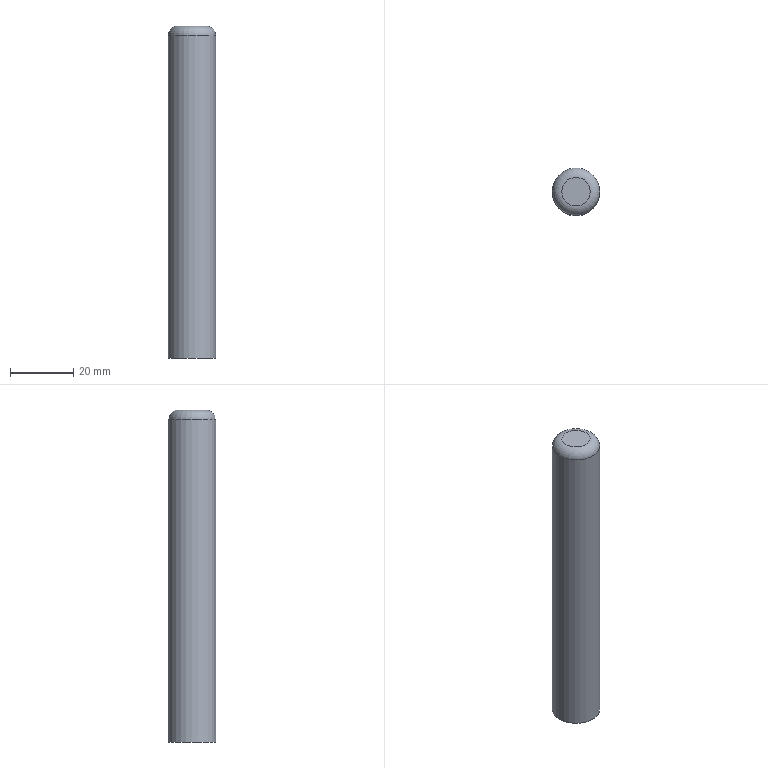Part | STEP file | Tube feed_id906_x_t | 1 solid | 4 faces | box 15 x 15 x 105 mm | volume 18472 mm3 | plane 2 | cylinder 1 | torus 1 | commonest cylinder face diameters 15 x1
STEP:
#1=CARTESIAN_POINT('',(0.,0.,0.));
#2=DIRECTION('',(0.,0.,1.));
#3=DIRECTION('',(1.,0.,0.));
#4=AXIS2_PLACEMENT_3D('',#1,#2,#3);
#5=CARTESIAN_POINT('',(-246.5,48.056,48.1));
#6=VERTEX_POINT('',#5);
#7=CARTESIAN_POINT('',(-261.5,48.056,48.1));
#8=VERTEX_POINT('',#7);
#9=CARTESIAN_POINT('',(-254.,48.056,48.1));
#10=DIRECTION('',(0.,0.,-1.));
#11=DIRECTION('',(1.,0.,0.));
#12=AXIS2_PLACEMENT_3D('',#9,#10,#11);
#13=CIRCLE('',#12,7.5);
#14=CARTESIAN_POINT('',(-254.,48.056,51.1));
#15=DIRECTION('',(0.,0.,-1.));
#16=DIRECTION('',(-1.,0.,0.));
#17=AXIS2_PLACEMENT_3D('',#14,#15,#16);
#18=CYLINDRICAL_SURFACE('',#17,7.5);
#19=CARTESIAN_POINT('',(3.142,3.));
#20=DIRECTION('',(1.,0.));
#21=VECTOR('',#20,1.);
#22=LINE('',#19,#21);
#23=(GEOMETRIC_REPRESENTATION_CONTEXT(2)PARAMETRIC_REPRESENTATION_CONTEXT()REPRESENTATION_CONTEXT('',''));
#24=DEFINITIONAL_REPRESENTATION('',(#22),#23);
#25=PCURVE('',#18,#24);
#26=CARTESIAN_POINT('',(-254.,48.056,48.1));
#27=DIRECTION('',(0.,0.,1.));
#28=DIRECTION('',(1.,0.,0.));
#29=AXIS2_PLACEMENT_3D('',#26,#27,#28);
#30=TOROIDAL_SURFACE('',#29,4.5,3.);
#31=CARTESIAN_POINT('',(6.283,6.283));
#32=DIRECTION('',(-1.,0.));
#33=VECTOR('',#32,1.);
#34=LINE('',#31,#33);
#35=(GEOMETRIC_REPRESENTATION_CONTEXT(2)PARAMETRIC_REPRESENTATION_CONTEXT()REPRESENTATION_CONTEXT('',''));
#36=DEFINITIONAL_REPRESENTATION('',(#34),#35);
#37=PCURVE('',#30,#36);
#38=SURFACE_CURVE('',#13,(#25,#37),.PCURVE_S1.);
#39=EDGE_CURVE('',#6,#8,#38,.T.);
#40=ORIENTED_EDGE('',*,*,#39,.T.);
#41=CARTESIAN_POINT('',(-261.5,48.056,-53.9));
#42=VERTEX_POINT('',#41);
#43=CARTESIAN_POINT('',(-261.5,48.056,48.1));
#44=CARTESIAN_POINT('',(-261.5,48.056,-53.9));
#45=B_SPLINE_CURVE_WITH_KNOTS('',1,(#43,#44),.UNSPECIFIED.,.F.,.F.,(2,2),(3.,105.),.PIECEWISE_BEZIER_KNOTS.);
#46=CARTESIAN_POINT('',(6.283,0.));
#47=DIRECTION('',(0.,1.));
#48=VECTOR('',#47,1.);
#49=LINE('',#46,#48);
#50=(GEOMETRIC_REPRESENTATION_CONTEXT(2)PARAMETRIC_REPRESENTATION_CONTEXT()REPRESENTATION_CONTEXT('',''));
#51=DEFINITIONAL_REPRESENTATION('',(#49),#50);
#52=PCURVE('',#18,#51);
#53=CARTESIAN_POINT('',(0.,0.));
#54=DIRECTION('',(0.,1.));
#55=VECTOR('',#54,1.);
#56=LINE('',#53,#55);
#57=(GEOMETRIC_REPRESENTATION_CONTEXT(2)PARAMETRIC_REPRESENTATION_CONTEXT()REPRESENTATION_CONTEXT('',''));
#58=DEFINITIONAL_REPRESENTATION('',(#56),#57);
#59=PCURVE('',#18,#58);
#60=SEAM_CURVE('',#45,(#52,#59),.PCURVE_S1.);
#61=EDGE_CURVE('',#8,#42,#60,.T.);
#62=ORIENTED_EDGE('',*,*,#61,.T.);
#63=CARTESIAN_POINT('',(-254.,48.056,-53.9));
#64=DIRECTION('',(0.,0.,1.));
#65=DIRECTION('',(-1.,0.,0.));
#66=AXIS2_PLACEMENT_3D('',#63,#64,#65);
#67=CIRCLE('',#66,7.5);
#68=CARTESIAN_POINT('',(6.283,105.));
#69=DIRECTION('',(-1.,0.));
#70=VECTOR('',#69,1.);
#71=LINE('',#68,#70);
#72=(GEOMETRIC_REPRESENTATION_CONTEXT(2)PARAMETRIC_REPRESENTATION_CONTEXT()REPRESENTATION_CONTEXT('',''));
#73=DEFINITIONAL_REPRESENTATION('',(#71),#72);
#74=PCURVE('',#18,#73);
#75=CARTESIAN_POINT('',(-254.,48.056,-53.9));
#76=DIRECTION('',(0.,0.,1.));
#77=DIRECTION('',(1.,0.,0.));
#78=AXIS2_PLACEMENT_3D('',#75,#76,#77);
#79=PLANE('',#78);
#80=CARTESIAN_POINT('',(0.,0.));
#81=DIRECTION('',(-1.,0.));
#82=AXIS2_PLACEMENT_2D('',#80,#81);
#83=CIRCLE('',#82,7.5);
#84=(GEOMETRIC_REPRESENTATION_CONTEXT(2)PARAMETRIC_REPRESENTATION_CONTEXT()REPRESENTATION_CONTEXT('',''));
#85=DEFINITIONAL_REPRESENTATION('',(#83),#84);
#86=PCURVE('',#79,#85);
#87=SURFACE_CURVE('',#67,(#74,#86),.PCURVE_S1.);
#88=EDGE_CURVE('',#42,#42,#87,.T.);
#89=ORIENTED_EDGE('',*,*,#88,.T.);
#90=ORIENTED_EDGE('',*,*,#61,.F.);
#91=CARTESIAN_POINT('',(-254.,48.056,48.1));
#92=DIRECTION('',(0.,0.,-1.));
#93=DIRECTION('',(1.,0.,0.));
#94=AXIS2_PLACEMENT_3D('',#91,#92,#93);
#95=CIRCLE('',#94,7.5);
#96=CARTESIAN_POINT('',(-3.142,3.));
#97=DIRECTION('',(1.,0.));
#98=VECTOR('',#97,1.);
#99=LINE('',#96,#98);
#100=(GEOMETRIC_REPRESENTATION_CONTEXT(2)PARAMETRIC_REPRESENTATION_CONTEXT()REPRESENTATION_CONTEXT('',''));
#101=DEFINITIONAL_REPRESENTATION('',(#99),#100);
#102=PCURVE('',#18,#101);
#103=CARTESIAN_POINT('',(6.283,6.283));
#104=DIRECTION('',(-1.,0.));
#105=VECTOR('',#104,1.);
#106=LINE('',#103,#105);
#107=(GEOMETRIC_REPRESENTATION_CONTEXT(2)PARAMETRIC_REPRESENTATION_CONTEXT()REPRESENTATION_CONTEXT('',''));
#108=DEFINITIONAL_REPRESENTATION('',(#106),#107);
#109=PCURVE('',#30,#108);
#110=SURFACE_CURVE('',#95,(#102,#109),.PCURVE_S1.);
#111=EDGE_CURVE('',#8,#6,#110,.T.);
#112=ORIENTED_EDGE('',*,*,#111,.T.);
#113=EDGE_LOOP('',(#40,#62,#89,#90,#112));
#114=FACE_BOUND('',#113,.T.);
#115=ADVANCED_FACE('',(#114),#18,.T.);
#116=CARTESIAN_POINT('',(-249.5,48.056,51.1));
#117=VERTEX_POINT('',#116);
#118=CARTESIAN_POINT('',(-254.,48.056,51.1));
#119=DIRECTION('',(0.,0.,1.));
#120=DIRECTION('',(1.,0.,0.));
#121=AXIS2_PLACEMENT_3D('',#118,#119,#120);
#122=CIRCLE('',#121,4.5);
#123=CARTESIAN_POINT('',(-254.,48.056,51.1));
#124=DIRECTION('',(0.,0.,1.));
#125=DIRECTION('',(1.,0.,0.));
#126=AXIS2_PLACEMENT_3D('',#123,#124,#125);
#127=PLANE('',#126);
#128=CARTESIAN_POINT('',(0.,0.));
#129=DIRECTION('',(1.,0.));
#130=AXIS2_PLACEMENT_2D('',#128,#129);
#131=CIRCLE('',#130,4.5);
#132=(GEOMETRIC_REPRESENTATION_CONTEXT(2)PARAMETRIC_REPRESENTATION_CONTEXT()REPRESENTATION_CONTEXT('',''));
#133=DEFINITIONAL_REPRESENTATION('',(#131),#132);
#134=PCURVE('',#127,#133);
#135=CARTESIAN_POINT('',(0.,7.854));
#136=DIRECTION('',(1.,0.));
#137=VECTOR('',#136,1.);
#138=LINE('',#135,#137);
#139=(GEOMETRIC_REPRESENTATION_CONTEXT(2)PARAMETRIC_REPRESENTATION_CONTEXT()REPRESENTATION_CONTEXT('',''));
#140=DEFINITIONAL_REPRESENTATION('',(#138),#139);
#141=PCURVE('',#30,#140);
#142=SURFACE_CURVE('',#122,(#134,#141),.PCURVE_S1.);
#143=EDGE_CURVE('',#117,#117,#142,.T.);
#144=ORIENTED_EDGE('',*,*,#143,.T.);
#145=EDGE_LOOP('',(#144));
#146=FACE_BOUND('',#145,.T.);
#147=ADVANCED_FACE('',(#146),#127,.T.);
#148=ORIENTED_EDGE('',*,*,#88,.F.);
#149=EDGE_LOOP('',(#148));
#150=FACE_BOUND('',#149,.T.);
#151=ADVANCED_FACE('',(#150),#79,.F.);
#152=ORIENTED_EDGE('',*,*,#39,.F.);
#153=CARTESIAN_POINT('',(-246.5,48.056,48.1));
#154=CARTESIAN_POINT('',(-246.5,48.056,48.902));
#155=CARTESIAN_POINT('',(-246.755,48.056,49.683));
#156=CARTESIAN_POINT('',(-247.244,48.056,50.356));
#157=CARTESIAN_POINT('',(-247.917,48.056,50.845));
#158=CARTESIAN_POINT('',(-248.698,48.056,51.1));
#159=CARTESIAN_POINT('',(-249.5,48.056,51.1));
#160=(BOUNDED_CURVE()B_SPLINE_CURVE(6,(#153,#154,#155,#156,#157,#158,#159),.UNSPECIFIED.,.F.,.F.)B_SPLINE_CURVE_WITH_KNOTS((7,7),(0.,1.571),.PIECEWISE_BEZIER_KNOTS.)CURVE()GEOMETRIC_REPRESENTATION_ITEM()RATIONAL_B_SPLINE_CURVE((1.031,1.01,0.9979,0.994,0.9979,1.01,1.031))REPRESENTATION_ITEM(''));
#161=CARTESIAN_POINT('',(6.283,6.283));
#162=DIRECTION('',(0.,1.));
#163=VECTOR('',#162,1.);
#164=LINE('',#161,#163);
#165=(GEOMETRIC_REPRESENTATION_CONTEXT(2)PARAMETRIC_REPRESENTATION_CONTEXT()REPRESENTATION_CONTEXT('',''));
#166=DEFINITIONAL_REPRESENTATION('',(#164),#165);
#167=PCURVE('',#30,#166);
#168=CARTESIAN_POINT('',(0.,6.283));
#169=DIRECTION('',(0.,1.));
#170=VECTOR('',#169,1.);
#171=LINE('',#168,#170);
#172=(GEOMETRIC_REPRESENTATION_CONTEXT(2)PARAMETRIC_REPRESENTATION_CONTEXT()REPRESENTATION_CONTEXT('',''));
#173=DEFINITIONAL_REPRESENTATION('',(#171),#172);
#174=PCURVE('',#30,#173);
#175=SEAM_CURVE('',#160,(#167,#174),.PCURVE_S1.);
#176=EDGE_CURVE('',#6,#117,#175,.T.);
#177=ORIENTED_EDGE('',*,*,#176,.T.);
#178=ORIENTED_EDGE('',*,*,#143,.F.);
#179=ORIENTED_EDGE('',*,*,#176,.F.);
#180=ORIENTED_EDGE('',*,*,#111,.F.);
#181=EDGE_LOOP('',(#152,#177,#178,#179,#180));
#182=FACE_BOUND('',#181,.T.);
#183=ADVANCED_FACE('',(#182),#30,.T.);
#184=CLOSED_SHELL('',(#115,#147,#151,#183));
#185=MANIFOLD_SOLID_BREP('',#184);
#186=(LENGTH_UNIT()NAMED_UNIT(*)SI_UNIT(.MILLI.,.METRE.));
#187=UNCERTAINTY_MEASURE_WITH_UNIT(LENGTH_MEASURE(0.00001),#186,'','');
#188=(NAMED_UNIT(*)PLANE_ANGLE_UNIT()SI_UNIT($,.RADIAN.));
#189=(NAMED_UNIT(*)SI_UNIT($,.STERADIAN.)SOLID_ANGLE_UNIT());
#190=(GEOMETRIC_REPRESENTATION_CONTEXT(3)GLOBAL_UNCERTAINTY_ASSIGNED_CONTEXT((#187))GLOBAL_UNIT_ASSIGNED_CONTEXT((#186,#188,#189))REPRESENTATION_CONTEXT('',''));
#191=ADVANCED_BREP_SHAPE_REPRESENTATION('',(#4,#185),#190);